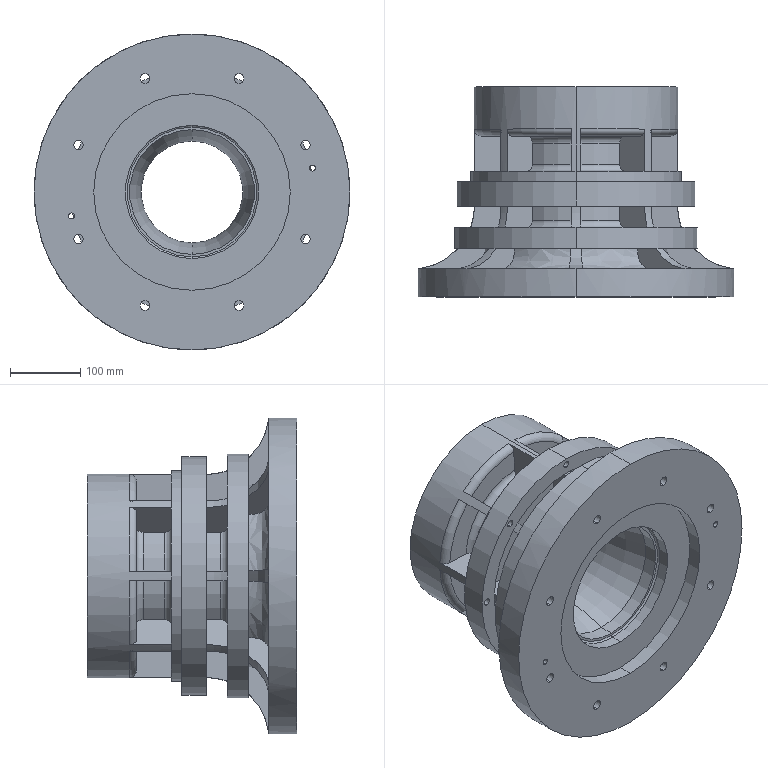Part | SolidWorks | features ICE 5, MirrorPattern 2, RevCut 2, Revolution 2, CirPattern 1 | 1 solid | 265 faces | box 450 x 299 x 450 mm | volume 13734208 mm3 | cylinder 94 | plane 91 | torus 68 | spline 8 | cone 4 | commonest cylinder face diameters 10 x16 13.5 x16 26 x16 185 x16 290 x10 145 x2